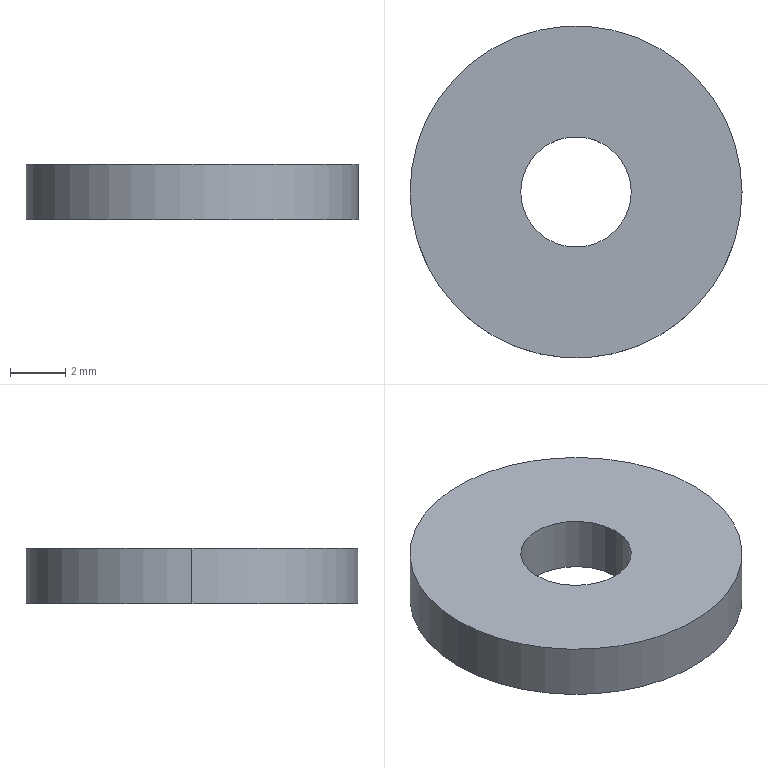Part | SolidWorks | features Extrusion 1 | 1 solid | 6 faces | box 12 x 12 x 2 mm | volume 201.062 mm3 | cylinder 4 | plane 2 | commonest cylinder face diameters 4 x2 12 x2
STEP:
#1=CARTESIAN_POINT('',(-2.,0.,2.));
#2=VERTEX_POINT('',#1);
#3=CARTESIAN_POINT('',(2.,0.,2.));
#4=VERTEX_POINT('',#3);
#5=CARTESIAN_POINT('',(0.,0.,2.));
#6=DIRECTION('',(0.,0.,1.));
#7=DIRECTION('',(1.,0.,0.));
#8=AXIS2_PLACEMENT_3D('',#5,#6,#7);
#9=CIRCLE('',#8,2.);
#10=EDGE_CURVE('',#2,#4,#9,.T.);
#11=ORIENTED_EDGE('',*,*,#10,.T.);
#12=CARTESIAN_POINT('',(2.,0.,0.));
#13=VERTEX_POINT('',#12);
#14=CARTESIAN_POINT('',(2.,0.,2.));
#15=DIRECTION('',(0.,0.,-1.));
#16=VECTOR('',#15,1000.);
#17=LINE('',#14,#16);
#18=EDGE_CURVE('',#4,#13,#17,.T.);
#19=ORIENTED_EDGE('',*,*,#18,.T.);
#20=CARTESIAN_POINT('',(-2.,0.,0.));
#21=VERTEX_POINT('',#20);
#22=CARTESIAN_POINT('',(0.,0.,0.));
#23=DIRECTION('',(0.,0.,1.));
#24=DIRECTION('',(1.,0.,0.));
#25=AXIS2_PLACEMENT_3D('',#22,#23,#24);
#26=CIRCLE('',#25,2.);
#27=EDGE_CURVE('',#21,#13,#26,.T.);
#28=ORIENTED_EDGE('',*,*,#27,.F.);
#29=CARTESIAN_POINT('',(-2.,0.,2.));
#30=DIRECTION('',(0.,0.,-1.));
#31=VECTOR('',#30,1000.);
#32=LINE('',#29,#31);
#33=EDGE_CURVE('',#2,#21,#32,.T.);
#34=ORIENTED_EDGE('',*,*,#33,.F.);
#35=EDGE_LOOP('',(#11,#19,#28,#34));
#36=FACE_OUTER_BOUND('',#35,.T.);
#37=CARTESIAN_POINT('',(0.,0.,2.));
#38=DIRECTION('',(0.,0.,-1.));
#39=DIRECTION('',(-1.,0.,0.));
#40=AXIS2_PLACEMENT_3D('',#37,#38,#39);
#41=CYLINDRICAL_SURFACE('',#40,2.);
#42=ADVANCED_FACE('',(#36),#41,.F.);
#43=CARTESIAN_POINT('',(6.,0.,2.));
#44=VERTEX_POINT('',#43);
#45=CARTESIAN_POINT('',(-6.,0.,2.));
#46=VERTEX_POINT('',#45);
#47=CARTESIAN_POINT('',(0.,0.,2.));
#48=DIRECTION('',(0.,0.,1.));
#49=DIRECTION('',(1.,0.,0.));
#50=AXIS2_PLACEMENT_3D('',#47,#48,#49);
#51=CIRCLE('',#50,6.);
#52=EDGE_CURVE('',#44,#46,#51,.T.);
#53=ORIENTED_EDGE('',*,*,#52,.F.);
#54=CARTESIAN_POINT('',(6.,0.,0.));
#55=VERTEX_POINT('',#54);
#56=CARTESIAN_POINT('',(6.,0.,2.));
#57=DIRECTION('',(0.,0.,-1.));
#58=VECTOR('',#57,1000.);
#59=LINE('',#56,#58);
#60=EDGE_CURVE('',#44,#55,#59,.T.);
#61=ORIENTED_EDGE('',*,*,#60,.T.);
#62=CARTESIAN_POINT('',(-6.,0.,0.));
#63=VERTEX_POINT('',#62);
#64=CARTESIAN_POINT('',(0.,0.,0.));
#65=DIRECTION('',(0.,0.,1.));
#66=DIRECTION('',(1.,0.,0.));
#67=AXIS2_PLACEMENT_3D('',#64,#65,#66);
#68=CIRCLE('',#67,6.);
#69=EDGE_CURVE('',#55,#63,#68,.T.);
#70=ORIENTED_EDGE('',*,*,#69,.T.);
#71=CARTESIAN_POINT('',(-6.,0.,2.));
#72=DIRECTION('',(0.,0.,-1.));
#73=VECTOR('',#72,1000.);
#74=LINE('',#71,#73);
#75=EDGE_CURVE('',#46,#63,#74,.T.);
#76=ORIENTED_EDGE('',*,*,#75,.F.);
#77=EDGE_LOOP('',(#53,#61,#70,#76));
#78=FACE_OUTER_BOUND('',#77,.T.);
#79=CARTESIAN_POINT('',(0.,0.,2.));
#80=DIRECTION('',(0.,0.,-1.));
#81=DIRECTION('',(-1.,0.,0.));
#82=AXIS2_PLACEMENT_3D('',#79,#80,#81);
#83=CYLINDRICAL_SURFACE('',#82,6.);
#84=ADVANCED_FACE('',(#78),#83,.T.);
#85=CARTESIAN_POINT('',(0.,0.,2.));
#86=DIRECTION('',(0.,0.,1.));
#87=DIRECTION('',(1.,0.,0.));
#88=AXIS2_PLACEMENT_3D('',#85,#86,#87);
#89=CIRCLE('',#88,6.);
#90=EDGE_CURVE('',#46,#44,#89,.T.);
#91=ORIENTED_EDGE('',*,*,#90,.T.);
#92=ORIENTED_EDGE('',*,*,#52,.T.);
#93=EDGE_LOOP('',(#91,#92));
#94=FACE_OUTER_BOUND('',#93,.T.);
#95=ORIENTED_EDGE('',*,*,#10,.F.);
#96=CARTESIAN_POINT('',(0.,0.,2.));
#97=DIRECTION('',(0.,0.,1.));
#98=DIRECTION('',(1.,0.,0.));
#99=AXIS2_PLACEMENT_3D('',#96,#97,#98);
#100=CIRCLE('',#99,2.);
#101=EDGE_CURVE('',#4,#2,#100,.T.);
#102=ORIENTED_EDGE('',*,*,#101,.F.);
#103=EDGE_LOOP('',(#95,#102));
#104=FACE_BOUND('',#103,.T.);
#105=CARTESIAN_POINT('',(0.,0.,2.));
#106=DIRECTION('',(0.,0.,1.));
#107=DIRECTION('',(1.,0.,0.));
#108=AXIS2_PLACEMENT_3D('',#105,#106,#107);
#109=PLANE('',#108);
#110=ADVANCED_FACE('',(#94,#104),#109,.T.);
#111=CARTESIAN_POINT('',(0.,0.,0.));
#112=DIRECTION('',(0.,0.,1.));
#113=DIRECTION('',(1.,0.,0.));
#114=AXIS2_PLACEMENT_3D('',#111,#112,#113);
#115=CIRCLE('',#114,6.);
#116=EDGE_CURVE('',#63,#55,#115,.T.);
#117=ORIENTED_EDGE('',*,*,#116,.F.);
#118=ORIENTED_EDGE('',*,*,#69,.F.);
#119=EDGE_LOOP('',(#117,#118));
#120=FACE_OUTER_BOUND('',#119,.T.);
#121=ORIENTED_EDGE('',*,*,#27,.T.);
#122=CARTESIAN_POINT('',(0.,0.,0.));
#123=DIRECTION('',(0.,0.,1.));
#124=DIRECTION('',(1.,0.,0.));
#125=AXIS2_PLACEMENT_3D('',#122,#123,#124);
#126=CIRCLE('',#125,2.);
#127=EDGE_CURVE('',#13,#21,#126,.T.);
#128=ORIENTED_EDGE('',*,*,#127,.T.);
#129=EDGE_LOOP('',(#121,#128));
#130=FACE_BOUND('',#129,.T.);
#131=CARTESIAN_POINT('',(0.,0.,0.));
#132=DIRECTION('',(0.,0.,1.));
#133=DIRECTION('',(1.,0.,0.));
#134=AXIS2_PLACEMENT_3D('',#131,#132,#133);
#135=PLANE('',#134);
#136=ADVANCED_FACE('',(#120,#130),#135,.F.);
#137=ORIENTED_EDGE('',*,*,#60,.F.);
#138=ORIENTED_EDGE('',*,*,#90,.F.);
#139=ORIENTED_EDGE('',*,*,#75,.T.);
#140=ORIENTED_EDGE('',*,*,#116,.T.);
#141=EDGE_LOOP('',(#137,#138,#139,#140));
#142=FACE_OUTER_BOUND('',#141,.T.);
#143=CARTESIAN_POINT('',(0.,0.,2.));
#144=DIRECTION('',(0.,0.,-1.));
#145=DIRECTION('',(-1.,0.,0.));
#146=AXIS2_PLACEMENT_3D('',#143,#144,#145);
#147=CYLINDRICAL_SURFACE('',#146,6.);
#148=ADVANCED_FACE('',(#142),#147,.T.);
#149=ORIENTED_EDGE('',*,*,#18,.F.);
#150=ORIENTED_EDGE('',*,*,#101,.T.);
#151=ORIENTED_EDGE('',*,*,#33,.T.);
#152=ORIENTED_EDGE('',*,*,#127,.F.);
#153=EDGE_LOOP('',(#149,#150,#151,#152));
#154=FACE_OUTER_BOUND('',#153,.T.);
#155=CARTESIAN_POINT('',(0.,0.,2.));
#156=DIRECTION('',(0.,0.,-1.));
#157=DIRECTION('',(-1.,0.,0.));
#158=AXIS2_PLACEMENT_3D('',#155,#156,#157);
#159=CYLINDRICAL_SURFACE('',#158,2.);
#160=ADVANCED_FACE('',(#154),#159,.F.);
#161=CLOSED_SHELL('',(#42,#84,#110,#136,#148,#160));
#162=MANIFOLD_SOLID_BREP('',#161);
#163=CARTESIAN_POINT('',(0.,0.,0.));
#164=DIRECTION('',(0.,0.,1.));
#165=DIRECTION('',(1.,0.,0.));
#166=AXIS2_PLACEMENT_3D('',#163,#164,#165);
#167=(LENGTH_UNIT()NAMED_UNIT(*)SI_UNIT(.MILLI.,.METRE.));
#168=UNCERTAINTY_MEASURE_WITH_UNIT(LENGTH_MEASURE(0.00001),#167,'','');
#169=(NAMED_UNIT(*)PLANE_ANGLE_UNIT()SI_UNIT($,.RADIAN.));
#170=(NAMED_UNIT(*)SI_UNIT($,.STERADIAN.)SOLID_ANGLE_UNIT());
#171=(GEOMETRIC_REPRESENTATION_CONTEXT(3)GLOBAL_UNCERTAINTY_ASSIGNED_CONTEXT((#168))GLOBAL_UNIT_ASSIGNED_CONTEXT((#167,#169,#170))REPRESENTATION_CONTEXT('',''));
#172=ADVANCED_BREP_SHAPE_REPRESENTATION('',(#162,#166),#171);